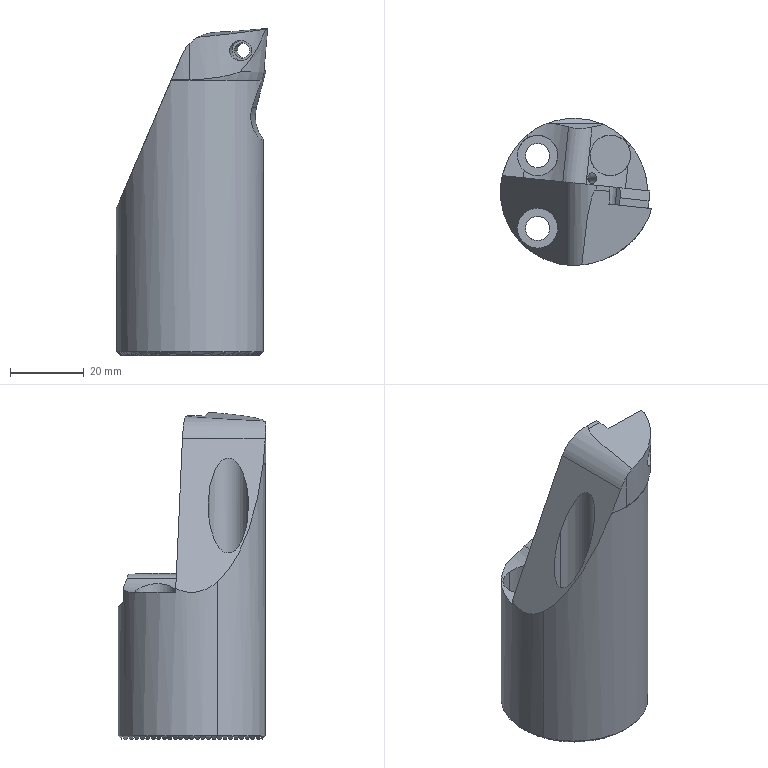CAM job | Mastercam | 3-axis milling, 5-axis milling, drilling
Tools:
tool_number,name,type,diameter_mm,corner_radius_mm,flutes,flute_length_mm,overall_length_mm,shoulder_length_mm,holder_diameter_mm,length_offset,diameter_offset,default_rpm,default_feed_mm_min,default_plunge_mm_min,coolant
1,2.8 Drill,drill,2.8,0,2,30,30,30,50,1,1,2143,257.16,600,COOL_OFF
1,12 Flat End Mill Rough,end mill,12,0,4,38,38,38,31.877,1,1,833,99.96,600,COOL_OFF
2,3.8 Drill,drill,3.8,0,2,25,50,40,50,2,2,1579,189.48,600,COOL_OFF
2,12 Flat End Mill Rough,end mill,12,0,4,38,38,38,31.877,2,2,833,99.96,600,COOL_OFF
3,10 Chamfer Mill,chamfer mill,10,0,4,25,75,30,50,3,3,2500,300,600,COOL_OFF
3,10 Chamfer Mill,chamfer mill,10,0,4,25,75,30,50,3,3,2500,300,600,COOL_OFF
3,10 Chamfer Mill,chamfer mill,10,0,4,25,75,30,50,3,3,2500,300,600,COOL_OFF
3,3 Drill,drill,3,0,2,50,65,50,50,3,3,2000,240,600,COOL_OFF
4,12 Flat End Mill Rough,end mill,12,0,4,38,38,38,31.877,4,4,833,99.96,600,COOL_OFF
4,6 Flat End Mill Rough,end mill,6,0,4,25,30,25,50,4,4,1667,200.04,600,COOL_OFF
4,11 Drill,drill,11,0,2,25,50,40,50,4,4,545,65.4,600,COOL_OFF
5,3 Flat End Mill Rough,end mill,3,0,4,22,24,22,27.495,5,5,3333,399.96,600,COOL_OFF
5,8 Flat End Mill Rough,end mill,8,0,4,25,25,25,50,5,5,1250,150,600,COOL_OFF
6,12 Flat End Mill Finish,end mill,12,0,4,35,35,35,31.877,6,6,833,99.96,600,COOL_OFF
6,8 Flat End Mill Finish,end mill,8,0,4,20,20,20,50,6,6,1250,150,600,COOL_OFF
7,3.3 Drill,drill,3.3,0,2,30,30,30,50,7,7,1818,218.16,600,COOL_OFF
7,4 Flat End Mill Finish,end mill,4,0,4,25,25,25,50,7,7,2500,300,600,COOL_OFF
7,4 Flat End Mill Finish,end mill,4,0,4,25,25,25,50,7,7,2500,300,600,COOL_OFF
7,6 Carbide Chamfer Mill,chamfer mill,6,0,4,25,30,30,50,7,7,4167,500.04,600,COOL_OFF
8,2 Taper Mill,tap,2,0,4,16.29,30,16.29,50,8,8,3000,360,600,COOL_OFF
8,26 60deg Thread cutter,thread mill,26,0,4,10,50,10,50,8,8,1923,230.76,600,COOL_OFF
9,30 Bull Nose Mill,bull end mill,30,0.8,4,30,100,50,50,9,9,400,48.0,600,COOL_OFF
9,12 Flat End Mill Finish,end mill,12,0,4,35,35,35,31.877,9,9,833,99.96,600,COOL_OFF
10,6 Chamfer Mill,chamfer mill,6,0,4,25,25,25,27.508,10,10,4167,500.04,600,COOL_OFF
10,50 Facing / Contour,end mill,50,0,4,5,50,18,50,10,10,1000,120,600,COOL_OFF
11,6.6 Drill,drill,6.6,0,2,25,50,40,50,11,11,909,109.08,600,COOL_OFF
11,4.2 Drill,drill,4.2,0,2,25,25,25,27.508,11,11,1428,171.36,600,COOL_OFF
12,10.8 Flat drill,drill,11,0,2,25,50,40,50,12,12,545,65.4,600,COOL_OFF
12,5.5 Flat End Mill,end mill,5.5,0,4,18,30,18,50,12,12,1819,218.28,600,COOL_OFF
13,2.5 Ball Mill,ball end mill,2.5,1.25,4,4,20,4,50,13,13,4800,576,600,COOL_OFF
13,11 Drill,drill,11,0,2,25,50,40,50,13,13,545,65.4,600,COOL_OFF
14,4.05 x 0.8 Thread Mill,thread mill,4.05,0,4,2.4,25,2.4,27.508,14,14,1481,177.72,600,COOL_OFF
14,5 Drill,drill,5,0,2,25,50,40,50,14,14,1200,144,600,COOL_OFF
14,5 Drill,drill,5,0,2,25,50,40,50,14,14,1200,144,600,COOL_OFF
14,5 Flat End Mill,end mill,5,0,4,20,20,20,50,14,14,2000,240,600,COOL_OFF
15,M6 x 1 RH Tap,drill,6,0,2,24,62,24,50,15,15,1000,1000,600,COOL_OFF
15,M6 x 1 RH Tap,drill,6,0,2,24,62,24,50,15,15,1000,1000,600,COOL_OFF
16,6 Flat End Mill,end mill,6,0,4,20,20,20,50,16,16,1667,200.04,600,COOL_OFF
Operations:
seq,operation,operation_type,tool_number,tool_name,tool_diameter_mm,spindle_rpm,feed_mm_min,plunge_mm_min,retract_mm_min,cycle_time_s,wcs,posted,nc_file
1,Contour (2D) - [WCS: Top] - [Tplane: 4XA0],Contour,10,50 Facing / Contour,50,1600,600,600,1200,11.942,Top,yes,3.nc
2,Contour (2D) - [WCS: Top] - [Tplane: 4XA0],Contour,2,12 Flat End Mill Rough,12,3500,400,2000,1200,28.411,Top,yes,3.nc
3,Drill/Counterbore - [WCS: Top] - [Tplane: 4XA0],Drill,3,3 Drill,3,2000,100,600,1200,11.8,Top,yes,3.nc
4,Peck Drill - [WCS: Top] - [Tplane: 4XA0],Drill,4,11 Drill,11,2000,80,600,1200,8.511,Top,yes,3.nc
5,Drill/Counterbore - [WCS: Top] - [Tplane: 4XA0],Drill,11,4.2 Drill,4.2,2300,60,600,1200,34.541,Top,yes,3.nc
6,Contour (2D chamfer) - [WCS: Top] - [Tplane: 4XA0],Contour,7,6 Carbide Chamfer Mill,6,3500,400,2000,1200,21.438,Top,yes,3.nc
7,Contour (2D chamfer) - [WCS: Top] - [Tplane: 4XA0],Contour,7,6 Carbide Chamfer Mill,6,3500,400,2000,1200,6.191,Top,yes,3.nc
8,Circle Mill - [WCS: Top] - [Tplane: 4XA0],CircleMill,5,8 Flat End Mill Rough,8,3500,400,2000,1200,7.513,Top,yes,3.nc
9,Circle Mill - [WCS: Top] - [Tplane: 4XA0],CircleMill,6,8 Flat End Mill Finish,8,3500,400,2000,1200,8.679,Top,yes,3.nc
10,Contour (2D) - [WCS: Top] - [Tplane: 4XA0],Contour,10,50 Facing / Contour,50,1600,600,600,1200,11.942,Top,yes,1.nc
11,Contour (2D) - [WCS: Top] - [Tplane: 4XA0],Contour,2,12 Flat End Mill Rough,12,3500,400,2000,1200,28.411,Top,yes,1.nc
12,Drill/Counterbore - [WCS: Top] - [Tplane: 4XA0],Drill,3,3 Drill,3,2000,100,600,1200,10.12,Top,yes,1.nc
13,Drill/Counterbore - [WCS: Top] - [Tplane: 4XA0],Drill,11,4.2 Drill,4.2,2300,60,600,1200,34.541,Top,yes,1.nc
14,Drill/Counterbore - [WCS: Top] - [Tplane: 4XA0],Drill,7,6 Carbide Chamfer Mill,6,2500,60,600,1200,8.499,Top,yes,1.nc
15,Peck Drill - [WCS: Top] - [Tplane: 4XA0],Drill,1,12 Flat End Mill Rough,12,2300,30,600,1200,62.621,Top,yes,1.nc
16,Contour (Ramp) - [WCS: Top] - [Tplane: 4XA0],Contour,16,6 Flat End Mill,6,4500,400,2000,1200,43.066,Top,yes,1.nc
17,Peck Drill - [WCS: Top] - [Tplane: 4XA0],Drill,4,11 Drill,11,2000,80,600,1200,8.364,Top,yes,1.nc
18,Contour (2D chamfer) - [WCS: Top] - [Tplane: 4XA0],Contour,7,6 Carbide Chamfer Mill,6,3500,400,2000,1200,21.438,Top,yes,1.nc
19,Contour (2D chamfer) - [WCS: Top] - [Tplane: 4XA0],Contour,7,6 Carbide Chamfer Mill,6,3500,400,2000,1200,6.191,Top,yes,1.nc
20,Circle Mill - [WCS: Top] - [Tplane: 4XA0],CircleMill,5,8 Flat End Mill Rough,8,3500,400,2000,1200,7.513,Top,yes,1.nc
21,Circle Mill - [WCS: Top] - [Tplane: 4XA0],CircleMill,6,8 Flat End Mill Finish,8,3500,400,2000,1200,8.679,Top,yes,1.nc
22,Contour (2D) - [WCS: Top] - [Tplane: 4XA0],Contour,10,50 Facing / Contour,50,1600,600,600,1200,11.942,Top,yes,3.nc
23,Contour (2D) - [WCS: Top] - [Tplane: 4XA0],Contour,2,12 Flat End Mill Rough,12,3500,400,2000,1200,28.411,Top,yes,3.nc
24,Drill/Counterbore - [WCS: Top] - [Tplane: 4XA0],Drill,3,3 Drill,3,2000,100,600,1200,10.12,Top,yes,3.nc
25,Drill/Counterbore - [WCS: Top] - [Tplane: 4XA0],Drill,11,4.2 Drill,4.2,2300,60,600,1200,34.541,Top,yes,3.nc
26,Peck Drill - [WCS: Top] - [Tplane: 4XA0],Drill,4,11 Drill,11,2000,80,600,1200,12.63,Top,yes,3.nc
27,Contour (2D chamfer) - [WCS: Top] - [Tplane: 4XA0],Contour,7,6 Carbide Chamfer Mill,6,3500,400,2000,1200,21.438,Top,yes,3.nc
28,Contour (2D chamfer) - [WCS: Top] - [Tplane: 4XA0],Contour,7,6 Carbide Chamfer Mill,6,3500,400,2000,1200,6.191,Top,yes,3.nc
29,Circle Mill - [WCS: Top] - [Tplane: 4XA0],CircleMill,5,8 Flat End Mill Rough,8,3500,400,2000,1200,7.513,Top,yes,3.nc
30,Circle Mill - [WCS: Top] - [Tplane: 4XA0],CircleMill,6,8 Flat End Mill Finish,8,3500,400,2000,1200,8.679,Top,yes,3.nc
31,Contour (2D) - [WCS: Top] - [Tplane: 2-A-90 Gear cutting],Contour,8,26 60deg Thread cutter,26,4000,1000,2000,1200,91.479,Top,yes,3.nc
32,Drill/Counterbore - [WCS: Top] - [Tplane: 4-A180],Drill,3,3 Drill,3,2000,100,600,1200,10.368,Top,yes,3.nc
33,Peck Drill - [WCS: Top] - [Tplane: 4-A180],Drill,13,11 Drill,11,2000,60,600,1200,106.219,Top,yes,3.nc
34,Drill/Counterbore - [WCS: Top] - [Tplane: 4-A180],Drill,12,5.5 Flat End Mill,5.5,800,60,600,1200,22.8,Top,yes,3.nc
35,Contour (2D) - [WCS: Top] - [Tplane: 2-A90 Fixture teeth],Contour,8,26 60deg Thread cutter,26,4000,1000,2000,1200,162.54,Top,yes,2.nc
36,Contour (Ramp) - [WCS: Top] - [Tplane: 4XFx],Contour,9,12 Flat End Mill Finish,12,3500,1500,2000,1200,11.202,Top,yes,2.nc
37,Contour (2D) - [WCS: Top] - [Tplane: 4XFx],Contour,9,12 Flat End Mill Finish,12,3500,600,2000,1200,5.024,Top,yes,2.nc
38,Drill/Counterbore - [WCS: Top] - [Tplane: Top],Drill,3,3 Drill,3,3000,300,600,1200,3.869,Top,yes,2.nc
39,Peck Drill - [WCS: Top] - [Tplane: Top],Drill,14,5 Flat End Mill,5,3000,300,600,1200,17.482,Top,yes,1.nc
40,Tap - [WCS: Top] - [Tplane: Top],Drill,15,M6 x 1 RH Tap,6,300,300,600,1200,43.306,Top,yes,1.nc
41,2D High Speed (2D Dynamic Mill) - [WCS: Top] - [Tplane: Top],HighSpeed2D,4,11 Drill,11,5500,4000,2000,1200,21.063,Top,yes,2.nc
42,Contour (2D) - [WCS: Top] - [Tplane: Top],Contour,9,12 Flat End Mill Finish,12,5500,600,2000,1200,15.277,Top,yes,2.nc
43,2D High Speed (2D Dynamic Mill) - [WCS: Top] - [Tplane: 1],HighSpeed2D,1,12 Flat End Mill Rough,12,3500,2800,2000,1200,200.974,Top,yes,4.nc
44,Contour (2D) - [WCS: Top] - [Tplane: 3- Hole-1],Contour,1,12 Flat End Mill Rough,12,3500,1500,2000,1200,3.126,Top,yes,4.nc
45,Drill/Counterbore - [WCS: Top] - [Tplane: 3-H],Drill,3,3 Drill,3,2000,20,600,1200,34.994,Top,yes,4.nc
46,Stock model - [WCS: Top] - [Tplane: 3-H] - 2_1,139,,,,0,0,0,0,0,Top,yes,1.nc|2.nc|3.nc|4.nc
47,2D High Speed (2D Dynamic Mill) - [WCS: Top] - [Tplane: 1],HighSpeed2D,1,12 Flat End Mill Rough,12,3500,2800,2000,1200,23.174,Top,yes,4.nc
48,Contour (2D) - [WCS: Top] - [Tplane: 1],Contour,1,12 Flat End Mill Rough,12,3500,1500,2000,1200,12.435,Top,yes,4.nc
49,Contour (2D) - [WCS: Top] - [Tplane: 1],Contour,1,12 Flat End Mill Rough,12,3500,600,2000,1200,14.343,Top,yes,4.nc
50,Contour (Ramp) - [WCS: Top] - [Tplane: 4],Contour,1,12 Flat End Mill Rough,12,3500,1500,2000,1200,5.563,Top,yes,4.nc
51,2D High Speed (2D Dynamic Mill) - [WCS: Top] - [Tplane: 2],HighSpeed2D,1,12 Flat End Mill Rough,12,3500,2800,2000,1200,83.891,Top,yes,4.nc
52,Contour (Ramp) - [WCS: Top] - [Tplane: 5],Contour,1,12 Flat End Mill Rough,12,3500,1500,2000,1200,7.488,Top,yes,4.nc
53,Contour (Ramp) - [WCS: Top] - [Tplane: 6],Contour,1,12 Flat End Mill Rough,12,3500,1500,2000,1200,5.421,Top,yes,4.nc
54,Contour (2D) - [WCS: Top] - [Tplane: 7],Contour,1,12 Flat End Mill Rough,12,3500,1500,2000,1200,11.461,Top,yes,4.nc
55,2D High Speed (2D Dynamic Mill) - [WCS: Top] - [Tplane: 1],HighSpeed2D,4,11 Drill,11,3500,1000,2000,1200,58.786,Top,yes,4.nc
56,Contour (2D) - [WCS: Top] - [Tplane: 8],Contour,1,12 Flat End Mill Rough,12,3500,1000,2000,1200,9.371,Top,yes,4.nc
57,Contour (Remachining) - [WCS: Top] - [Tplane: 1],Contour,5,8 Flat End Mill Rough,8,3500,400,2000,1200,64.448,Top,yes,4.nc
58,Contour (2D) - [WCS: Top] - [Tplane: 8],Contour,6,8 Flat End Mill Finish,8,3500,600,2000,1200,13.271,Top,yes,4.nc
59,Contour (2D) - [WCS: Top] - [Tplane: 1],Contour,7,6 Carbide Chamfer Mill,6,3500,400,2000,1200,13.483,Top,yes,4.nc
60,Contour (2D) - [WCS: Top] - [Tplane: 1],Contour,8,26 60deg Thread cutter,26,3000,360,600,1200,16.778,Top,yes,4.nc
61,Contour (2D) - [WCS: Top] - [Tplane: 1],Contour,6,8 Flat End Mill Finish,8,3000,600,2000,1200,7.135,Top,yes,4.nc
62,Contour (2D) - [WCS: Top] - [Tplane: 4],Contour,6,8 Flat End Mill Finish,8,3500,600,2000,1200,4.175,Top,yes,4.nc
63,Contour (2D) - [WCS: Top] - [Tplane: 5],Contour,6,8 Flat End Mill Finish,8,3500,600,2000,1200,3.911,Top,yes,4.nc
64,Contour (2D) - [WCS: Top] - [Tplane: 6],Contour,6,8 Flat End Mill Finish,8,3500,600,2000,1200,3.553,Top,yes,4.nc
65,Contour (2D) - [WCS: Top] - [Tplane: 7],Contour,6,8 Flat End Mill Finish,8,3500,600,2000,1200,10.654,Top,yes,4.nc
66,Contour (2D) - [WCS: Top] - [Tplane: 2],Contour,6,8 Flat End Mill Finish,8,3000,600,2000,1200,22.399,Top,yes,4.nc
67,Contour (2D) - [WCS: Top] - [Tplane: 1],Contour,6,8 Flat End Mill Finish,8,3500,600,2000,1200,4.747,Top,yes,4.nc
68,Contour (2D) - [WCS: Top] - [Tplane: 1],Contour,9,12 Flat End Mill Finish,12,1500,500,2000,1200,21.062,Top,yes,4.nc
69,Contour (2D) - [WCS: Top] - [Tplane: 1],Contour,9,12 Flat End Mill Finish,12,1500,500,2000,1200,20.084,Top,yes,4.nc
70,Drill/Counterbore - [WCS: Top] - [Tplane: 1],Drill,10,50 Facing / Contour,50,3000,100,600,1200,1.677,Top,yes,4.nc
71,Drill/Counterbore - [WCS: Top] - [Tplane: 1],Drill,11,4.2 Drill,4.2,2500,70,600,1200,12.535,Top,yes,4.nc
72,Drill/Counterbore - [WCS: Top] - [Tplane: 1],Drill,10,50 Facing / Contour,50,2000,100,600,1200,2.766,Top,yes,4.nc
73,Stock model - [WCS: Top] - [Tplane: 3-H] - 2,139,,,,0,0,0,0,0,Top,yes,1.nc|2.nc|3.nc|4.nc
74,Drill/Counterbore - [WCS: Top] - [Tplane: 9-CB],Drill,12,5.5 Flat End Mill,5.5,2000,40,600,1200,10.249,Top,yes,4.nc
75,Thread Mill - [WCS: Top] - [Tplane: 1],ThreadMill,14,5 Flat End Mill,5,2000,70,600,1200,83.753,Top,yes,4.nc
76,Deburr 5-axis - [WCS: Top] - [Tplane: Top],459,13,11 Drill,11,6000,600,2000,1200,17.199,Top,yes,4.nc
77,Deburr 5-axis - [WCS: Top] - [Tplane: Top],459,13,11 Drill,11,6000,600,2000,1200,4.529,Top,yes,4.nc
78,Drill/Counterbore - [WCS: Top] - [Tplane: Top],Drill,3,3 Drill,3,3000,300,600,1200,3.869,Top,yes,4.nc
79,Drill/Counterbore - [WCS: Top] - [Tplane: Top],Drill,14,5 Flat End Mill,5,3000,300,600,1200,14.314,Top,yes,4.nc
80,Misc. #2 - [WCS: Top] - [Tplane: Top],Drill,15,M6 x 1 RH Tap,6,300,300,600,1200,8.17,Top,yes,4.nc